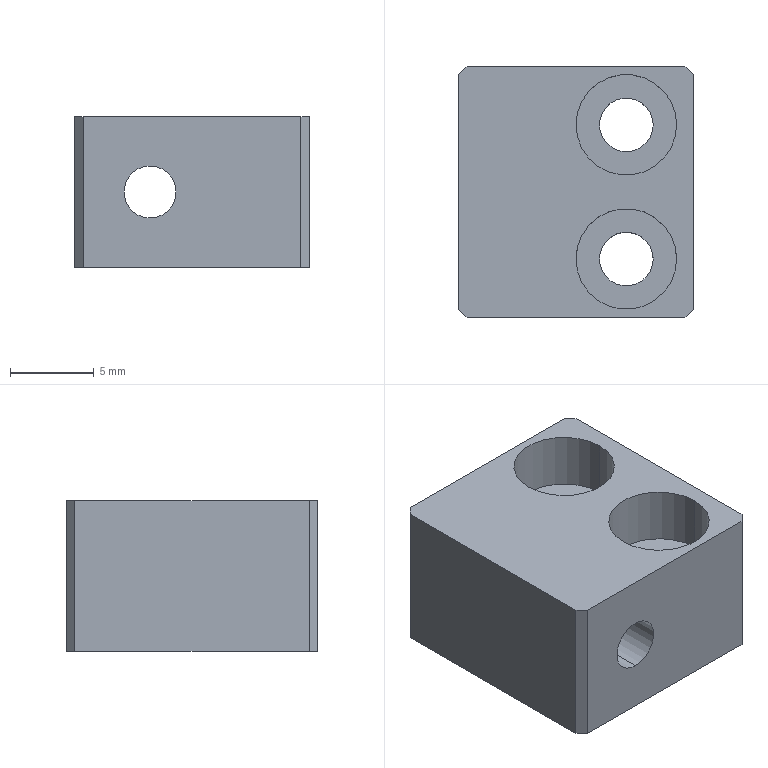Part | STEP file | PN_0021 Mount electronic clip pressure block | 1 solid | 22 faces | box 14 x 15 x 9 mm | volume 1490 mm3 | plane 12 | cylinder 10 | commonest cylinder face diameters 3.2 x4 6 x4 3.1 x2